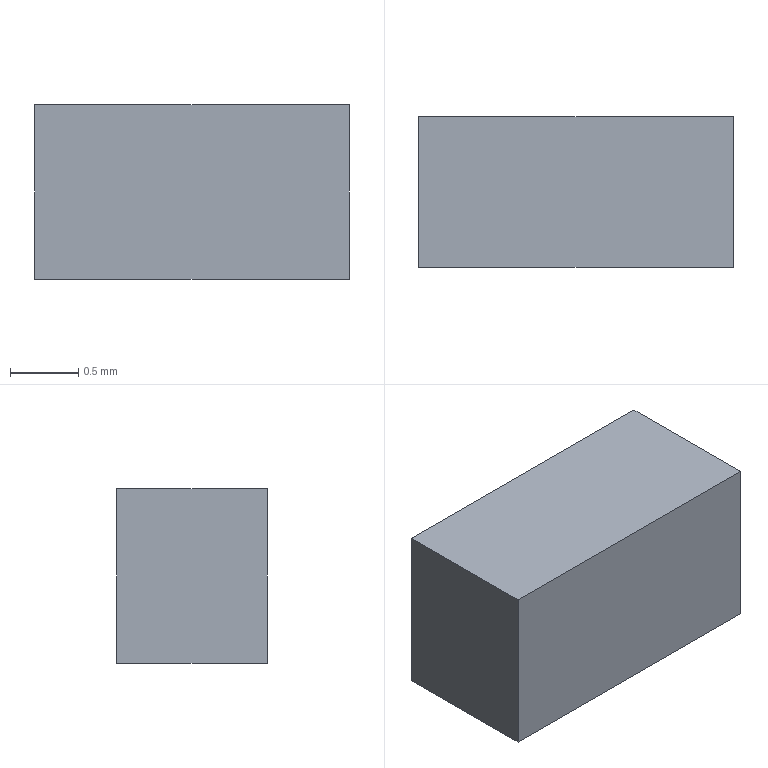Part | Creo | 1 solid | 6 faces | box 2.3 x 1.1 x 1.275 mm | volume 3.225 mm3 | plane 6
STEP:
#1=CARTESIAN_POINT('',(0.,0.,0.));
#2=DIRECTION('',(0.,0.,1.));
#3=DIRECTION('',(1.,0.,0.));
#4=AXIS2_PLACEMENT_3D('',#1,#2,#3);
#5=CARTESIAN_POINT('',(-1.15,0.55,0.));
#6=VERTEX_POINT('',#5);
#7=CARTESIAN_POINT('',(-1.15,-0.55,0.));
#8=VERTEX_POINT('',#7);
#9=CARTESIAN_POINT('',(-1.15,0.55,0.));
#10=DIRECTION('',(0.,-1.,0.));
#11=VECTOR('',#10,1.1);
#12=LINE('',#9,#11);
#13=EDGE_CURVE('',#6,#8,#12,.T.);
#14=ORIENTED_EDGE('',*,*,#13,.T.);
#15=CARTESIAN_POINT('',(1.15,-0.55,0.));
#16=VERTEX_POINT('',#15);
#17=CARTESIAN_POINT('',(-1.15,-0.55,0.));
#18=DIRECTION('',(1.,0.,0.));
#19=VECTOR('',#18,2.3);
#20=LINE('',#17,#19);
#21=EDGE_CURVE('',#8,#16,#20,.T.);
#22=ORIENTED_EDGE('',*,*,#21,.T.);
#23=CARTESIAN_POINT('',(1.15,0.55,0.));
#24=VERTEX_POINT('',#23);
#25=CARTESIAN_POINT('',(1.15,-0.55,0.));
#26=DIRECTION('',(0.,1.,0.));
#27=VECTOR('',#26,1.1);
#28=LINE('',#25,#27);
#29=EDGE_CURVE('',#16,#24,#28,.T.);
#30=ORIENTED_EDGE('',*,*,#29,.T.);
#31=CARTESIAN_POINT('',(1.15,0.55,0.));
#32=DIRECTION('',(-1.,0.,0.));
#33=VECTOR('',#32,2.3);
#34=LINE('',#31,#33);
#35=EDGE_CURVE('',#24,#6,#34,.T.);
#36=ORIENTED_EDGE('',*,*,#35,.T.);
#37=EDGE_LOOP('',(#14,#22,#30,#36));
#38=FACE_OUTER_BOUND('',#37,.F.);
#39=CARTESIAN_POINT('',(0.,0.,0.));
#40=DIRECTION('',(0.,0.,1.));
#41=DIRECTION('',(1.,0.,0.));
#42=AXIS2_PLACEMENT_3D('',#39,#40,#41);
#43=PLANE('',#42);
#44=ADVANCED_FACE('',(#38),#43,.F.);
#45=ORIENTED_EDGE('',*,*,#13,.F.);
#46=CARTESIAN_POINT('',(-1.15,0.55,1.275));
#47=VERTEX_POINT('',#46);
#48=CARTESIAN_POINT('',(-1.15,0.55,0.));
#49=DIRECTION('',(0.,0.,1.));
#50=VECTOR('',#49,1.275);
#51=LINE('',#48,#50);
#52=EDGE_CURVE('',#6,#47,#51,.T.);
#53=ORIENTED_EDGE('',*,*,#52,.T.);
#54=CARTESIAN_POINT('',(-1.15,-0.55,1.275));
#55=VERTEX_POINT('',#54);
#56=CARTESIAN_POINT('',(-1.15,0.55,1.275));
#57=DIRECTION('',(0.,-1.,0.));
#58=VECTOR('',#57,1.1);
#59=LINE('',#56,#58);
#60=EDGE_CURVE('',#47,#55,#59,.T.);
#61=ORIENTED_EDGE('',*,*,#60,.T.);
#62=CARTESIAN_POINT('',(-1.15,-0.55,0.));
#63=DIRECTION('',(0.,0.,1.));
#64=VECTOR('',#63,1.275);
#65=LINE('',#62,#64);
#66=EDGE_CURVE('',#8,#55,#65,.T.);
#67=ORIENTED_EDGE('',*,*,#66,.F.);
#68=EDGE_LOOP('',(#45,#53,#61,#67));
#69=FACE_OUTER_BOUND('',#68,.F.);
#70=CARTESIAN_POINT('',(-1.15,0.55,0.));
#71=DIRECTION('',(-1.,0.,0.));
#72=DIRECTION('',(0.,-1.,0.));
#73=AXIS2_PLACEMENT_3D('',#70,#71,#72);
#74=PLANE('',#73);
#75=ADVANCED_FACE('',(#69),#74,.T.);
#76=ORIENTED_EDGE('',*,*,#35,.F.);
#77=CARTESIAN_POINT('',(1.15,0.55,1.275));
#78=VERTEX_POINT('',#77);
#79=CARTESIAN_POINT('',(1.15,0.55,0.));
#80=DIRECTION('',(0.,0.,1.));
#81=VECTOR('',#80,1.275);
#82=LINE('',#79,#81);
#83=EDGE_CURVE('',#24,#78,#82,.T.);
#84=ORIENTED_EDGE('',*,*,#83,.T.);
#85=CARTESIAN_POINT('',(1.15,0.55,1.275));
#86=DIRECTION('',(-1.,0.,0.));
#87=VECTOR('',#86,2.3);
#88=LINE('',#85,#87);
#89=EDGE_CURVE('',#78,#47,#88,.T.);
#90=ORIENTED_EDGE('',*,*,#89,.T.);
#91=ORIENTED_EDGE('',*,*,#52,.F.);
#92=EDGE_LOOP('',(#76,#84,#90,#91));
#93=FACE_OUTER_BOUND('',#92,.F.);
#94=CARTESIAN_POINT('',(1.15,0.55,0.));
#95=DIRECTION('',(0.,1.,0.));
#96=DIRECTION('',(-1.,0.,0.));
#97=AXIS2_PLACEMENT_3D('',#94,#95,#96);
#98=PLANE('',#97);
#99=ADVANCED_FACE('',(#93),#98,.T.);
#100=ORIENTED_EDGE('',*,*,#29,.F.);
#101=CARTESIAN_POINT('',(1.15,-0.55,1.275));
#102=VERTEX_POINT('',#101);
#103=CARTESIAN_POINT('',(1.15,-0.55,0.));
#104=DIRECTION('',(0.,0.,1.));
#105=VECTOR('',#104,1.275);
#106=LINE('',#103,#105);
#107=EDGE_CURVE('',#16,#102,#106,.T.);
#108=ORIENTED_EDGE('',*,*,#107,.T.);
#109=CARTESIAN_POINT('',(1.15,-0.55,1.275));
#110=DIRECTION('',(0.,1.,0.));
#111=VECTOR('',#110,1.1);
#112=LINE('',#109,#111);
#113=EDGE_CURVE('',#102,#78,#112,.T.);
#114=ORIENTED_EDGE('',*,*,#113,.T.);
#115=ORIENTED_EDGE('',*,*,#83,.F.);
#116=EDGE_LOOP('',(#100,#108,#114,#115));
#117=FACE_OUTER_BOUND('',#116,.F.);
#118=CARTESIAN_POINT('',(1.15,-0.55,0.));
#119=DIRECTION('',(1.,0.,0.));
#120=DIRECTION('',(0.,1.,0.));
#121=AXIS2_PLACEMENT_3D('',#118,#119,#120);
#122=PLANE('',#121);
#123=ADVANCED_FACE('',(#117),#122,.T.);
#124=ORIENTED_EDGE('',*,*,#21,.F.);
#125=ORIENTED_EDGE('',*,*,#66,.T.);
#126=CARTESIAN_POINT('',(-1.15,-0.55,1.275));
#127=DIRECTION('',(1.,0.,0.));
#128=VECTOR('',#127,2.3);
#129=LINE('',#126,#128);
#130=EDGE_CURVE('',#55,#102,#129,.T.);
#131=ORIENTED_EDGE('',*,*,#130,.T.);
#132=ORIENTED_EDGE('',*,*,#107,.F.);
#133=EDGE_LOOP('',(#124,#125,#131,#132));
#134=FACE_OUTER_BOUND('',#133,.F.);
#135=CARTESIAN_POINT('',(-1.15,-0.55,0.));
#136=DIRECTION('',(0.,-1.,0.));
#137=DIRECTION('',(1.,0.,0.));
#138=AXIS2_PLACEMENT_3D('',#135,#136,#137);
#139=PLANE('',#138);
#140=ADVANCED_FACE('',(#134),#139,.T.);
#141=ORIENTED_EDGE('',*,*,#60,.F.);
#142=ORIENTED_EDGE('',*,*,#89,.F.);
#143=ORIENTED_EDGE('',*,*,#113,.F.);
#144=ORIENTED_EDGE('',*,*,#130,.F.);
#145=EDGE_LOOP('',(#141,#142,#143,#144));
#146=FACE_OUTER_BOUND('',#145,.F.);
#147=CARTESIAN_POINT('',(0.,0.,1.275));
#148=DIRECTION('',(0.,0.,1.));
#149=DIRECTION('',(1.,0.,0.));
#150=AXIS2_PLACEMENT_3D('',#147,#148,#149);
#151=PLANE('',#150);
#152=ADVANCED_FACE('',(#146),#151,.T.);
#153=CLOSED_SHELL('',(#44,#75,#99,#123,#140,#152));
#154=MANIFOLD_SOLID_BREP('',#153);
#155=(LENGTH_UNIT()NAMED_UNIT(*)SI_UNIT(.MILLI.,.METRE.));
#156=UNCERTAINTY_MEASURE_WITH_UNIT(LENGTH_MEASURE(0.000285),#155,'','');
#157=(NAMED_UNIT(*)PLANE_ANGLE_UNIT()SI_UNIT($,.RADIAN.));
#158=PLANE_ANGLE_MEASURE_WITH_UNIT(PLANE_ANGLE_MEASURE(0.01745),#157);
#159=(CONVERSION_BASED_UNIT('DEGREE',#158)NAMED_UNIT(*)PLANE_ANGLE_UNIT());
#160=(NAMED_UNIT(*)SI_UNIT($,.STERADIAN.)SOLID_ANGLE_UNIT());
#161=(GEOMETRIC_REPRESENTATION_CONTEXT(3)GLOBAL_UNCERTAINTY_ASSIGNED_CONTEXT((#156))GLOBAL_UNIT_ASSIGNED_CONTEXT((#155,#159,#160))REPRESENTATION_CONTEXT('',''));
#162=ADVANCED_BREP_SHAPE_REPRESENTATION('',(#4,#154),#161);